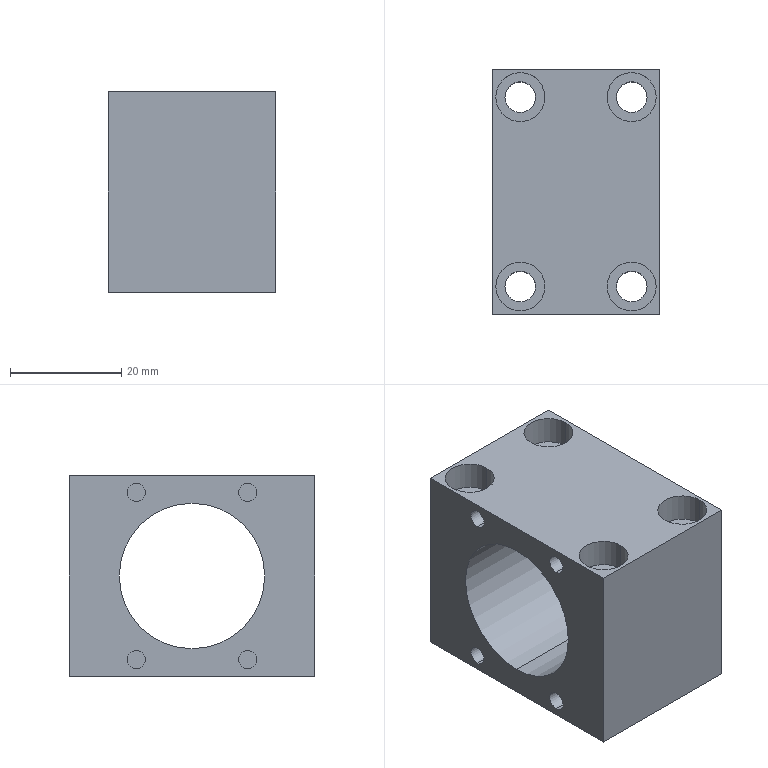Part | SolidWorks | features BaseBody 1 | 1 solid | 52 faces | box 30 x 44 x 36 mm | volume 26457 mm3 | cylinder 34 | plane 18 | commonest cylinder face diameters 3.3 x16 5.5 x8 8.8 x8 26.1 x2
STEP:
#1=CARTESIAN_POINT('',(-15.,0.,31.05));
#2=VERTEX_POINT('',#1);
#3=CARTESIAN_POINT('',(-15.,0.,4.95));
#4=VERTEX_POINT('',#3);
#5=CARTESIAN_POINT('',(-15.,0.,18.));
#6=DIRECTION('',(1.,0.,0.));
#7=DIRECTION('',(0.,0.,-1.));
#8=AXIS2_PLACEMENT_3D('',#5,#6,#7);
#9=CIRCLE('',#8,13.05);
#10=EDGE_CURVE('',#2,#4,#9,.T.);
#11=ORIENTED_EDGE('',*,*,#10,.F.);
#12=CARTESIAN_POINT('',(15.,0.,31.05));
#13=VERTEX_POINT('',#12);
#14=CARTESIAN_POINT('',(-16.,0.,31.05));
#15=DIRECTION('',(1.,0.,0.));
#16=VECTOR('',#15,1000.);
#17=LINE('',#14,#16);
#18=EDGE_CURVE('',#2,#13,#17,.T.);
#19=ORIENTED_EDGE('',*,*,#18,.T.);
#20=CARTESIAN_POINT('',(15.,0.,4.95));
#21=VERTEX_POINT('',#20);
#22=CARTESIAN_POINT('',(15.,0.,18.));
#23=DIRECTION('',(-1.,0.,0.));
#24=DIRECTION('',(0.,0.,-1.));
#25=AXIS2_PLACEMENT_3D('',#22,#23,#24);
#26=CIRCLE('',#25,13.05);
#27=EDGE_CURVE('',#21,#13,#26,.T.);
#28=ORIENTED_EDGE('',*,*,#27,.F.);
#29=CARTESIAN_POINT('',(-16.,0.,4.95));
#30=DIRECTION('',(1.,0.,0.));
#31=VECTOR('',#30,1000.);
#32=LINE('',#29,#31);
#33=EDGE_CURVE('',#4,#21,#32,.T.);
#34=ORIENTED_EDGE('',*,*,#33,.F.);
#35=EDGE_LOOP('',(#11,#19,#28,#34));
#36=FACE_OUTER_BOUND('',#35,.T.);
#37=CARTESIAN_POINT('',(-16.,0.,18.));
#38=DIRECTION('',(1.,0.,0.));
#39=DIRECTION('',(0.,0.,-1.));
#40=AXIS2_PLACEMENT_3D('',#37,#38,#39);
#41=CYLINDRICAL_SURFACE('',#40,13.05);
#42=ADVANCED_FACE('',(#36),#41,.F.);
#43=CARTESIAN_POINT('',(-2.8,-10.,31.35));
#44=VERTEX_POINT('',#43);
#45=CARTESIAN_POINT('',(-2.8,-10.,34.65));
#46=VERTEX_POINT('',#45);
#47=CARTESIAN_POINT('',(-2.8,-10.,33.));
#48=DIRECTION('',(-1.,0.,0.));
#49=DIRECTION('',(0.,0.,1.));
#50=AXIS2_PLACEMENT_3D('',#47,#48,#49);
#51=CIRCLE('',#50,1.65);
#52=EDGE_CURVE('',#44,#46,#51,.T.);
#53=ORIENTED_EDGE('',*,*,#52,.F.);
#54=CARTESIAN_POINT('',(-15.,-10.,31.35));
#55=VERTEX_POINT('',#54);
#56=CARTESIAN_POINT('',(-2.8,-10.,31.35));
#57=DIRECTION('',(-1.,0.,0.));
#58=VECTOR('',#57,1000.);
#59=LINE('',#56,#58);
#60=EDGE_CURVE('',#44,#55,#59,.T.);
#61=ORIENTED_EDGE('',*,*,#60,.T.);
#62=CARTESIAN_POINT('',(-15.,-10.,34.65));
#63=VERTEX_POINT('',#62);
#64=CARTESIAN_POINT('',(-15.,-10.,33.));
#65=DIRECTION('',(-1.,0.,0.));
#66=DIRECTION('',(0.,0.,1.));
#67=AXIS2_PLACEMENT_3D('',#64,#65,#66);
#68=CIRCLE('',#67,1.65);
#69=EDGE_CURVE('',#55,#63,#68,.T.);
#70=ORIENTED_EDGE('',*,*,#69,.T.);
#71=CARTESIAN_POINT('',(-2.8,-10.,34.65));
#72=DIRECTION('',(-1.,0.,0.));
#73=VECTOR('',#72,1000.);
#74=LINE('',#71,#73);
#75=EDGE_CURVE('',#46,#63,#74,.T.);
#76=ORIENTED_EDGE('',*,*,#75,.F.);
#77=EDGE_LOOP('',(#53,#61,#70,#76));
#78=FACE_OUTER_BOUND('',#77,.T.);
#79=CARTESIAN_POINT('',(-2.8,-10.,33.));
#80=DIRECTION('',(-1.,0.,0.));
#81=DIRECTION('',(0.,0.,1.));
#82=AXIS2_PLACEMENT_3D('',#79,#80,#81);
#83=CYLINDRICAL_SURFACE('',#82,1.65);
#84=ADVANCED_FACE('',(#78),#83,.F.);
#85=CARTESIAN_POINT('',(-2.8,-10.,1.35));
#86=VERTEX_POINT('',#85);
#87=CARTESIAN_POINT('',(-2.8,-10.,4.65));
#88=VERTEX_POINT('',#87);
#89=CARTESIAN_POINT('',(-2.8,-10.,3.));
#90=DIRECTION('',(-1.,0.,0.));
#91=DIRECTION('',(0.,0.,1.));
#92=AXIS2_PLACEMENT_3D('',#89,#90,#91);
#93=CIRCLE('',#92,1.65);
#94=EDGE_CURVE('',#86,#88,#93,.T.);
#95=ORIENTED_EDGE('',*,*,#94,.F.);
#96=CARTESIAN_POINT('',(-15.,-10.,1.35));
#97=VERTEX_POINT('',#96);
#98=CARTESIAN_POINT('',(-2.8,-10.,1.35));
#99=DIRECTION('',(-1.,0.,0.));
#100=VECTOR('',#99,1000.);
#101=LINE('',#98,#100);
#102=EDGE_CURVE('',#86,#97,#101,.T.);
#103=ORIENTED_EDGE('',*,*,#102,.T.);
#104=CARTESIAN_POINT('',(-15.,-10.,4.65));
#105=VERTEX_POINT('',#104);
#106=CARTESIAN_POINT('',(-15.,-10.,3.));
#107=DIRECTION('',(-1.,0.,0.));
#108=DIRECTION('',(0.,0.,1.));
#109=AXIS2_PLACEMENT_3D('',#106,#107,#108);
#110=CIRCLE('',#109,1.65);
#111=EDGE_CURVE('',#97,#105,#110,.T.);
#112=ORIENTED_EDGE('',*,*,#111,.T.);
#113=CARTESIAN_POINT('',(-2.8,-10.,4.65));
#114=DIRECTION('',(-1.,0.,0.));
#115=VECTOR('',#114,1000.);
#116=LINE('',#113,#115);
#117=EDGE_CURVE('',#88,#105,#116,.T.);
#118=ORIENTED_EDGE('',*,*,#117,.F.);
#119=EDGE_LOOP('',(#95,#103,#112,#118));
#120=FACE_OUTER_BOUND('',#119,.T.);
#121=CARTESIAN_POINT('',(-2.8,-10.,3.));
#122=DIRECTION('',(-1.,0.,0.));
#123=DIRECTION('',(0.,0.,1.));
#124=AXIS2_PLACEMENT_3D('',#121,#122,#123);
#125=CYLINDRICAL_SURFACE('',#124,1.65);
#126=ADVANCED_FACE('',(#120),#125,.F.);
#127=CARTESIAN_POINT('',(-2.8,10.,31.35));
#128=VERTEX_POINT('',#127);
#129=CARTESIAN_POINT('',(-2.8,10.,34.65));
#130=VERTEX_POINT('',#129);
#131=CARTESIAN_POINT('',(-2.8,10.,33.));
#132=DIRECTION('',(-1.,0.,0.));
#133=DIRECTION('',(0.,0.,1.));
#134=AXIS2_PLACEMENT_3D('',#131,#132,#133);
#135=CIRCLE('',#134,1.65);
#136=EDGE_CURVE('',#128,#130,#135,.T.);
#137=ORIENTED_EDGE('',*,*,#136,.F.);
#138=CARTESIAN_POINT('',(-15.,10.,31.35));
#139=VERTEX_POINT('',#138);
#140=CARTESIAN_POINT('',(-2.8,10.,31.35));
#141=DIRECTION('',(-1.,0.,0.));
#142=VECTOR('',#141,1000.);
#143=LINE('',#140,#142);
#144=EDGE_CURVE('',#128,#139,#143,.T.);
#145=ORIENTED_EDGE('',*,*,#144,.T.);
#146=CARTESIAN_POINT('',(-15.,10.,34.65));
#147=VERTEX_POINT('',#146);
#148=CARTESIAN_POINT('',(-15.,10.,33.));
#149=DIRECTION('',(-1.,0.,0.));
#150=DIRECTION('',(0.,0.,1.));
#151=AXIS2_PLACEMENT_3D('',#148,#149,#150);
#152=CIRCLE('',#151,1.65);
#153=EDGE_CURVE('',#139,#147,#152,.T.);
#154=ORIENTED_EDGE('',*,*,#153,.T.);
#155=CARTESIAN_POINT('',(-2.8,10.,34.65));
#156=DIRECTION('',(-1.,0.,0.));
#157=VECTOR('',#156,1000.);
#158=LINE('',#155,#157);
#159=EDGE_CURVE('',#130,#147,#158,.T.);
#160=ORIENTED_EDGE('',*,*,#159,.F.);
#161=EDGE_LOOP('',(#137,#145,#154,#160));
#162=FACE_OUTER_BOUND('',#161,.T.);
#163=CARTESIAN_POINT('',(-2.8,10.,33.));
#164=DIRECTION('',(-1.,0.,0.));
#165=DIRECTION('',(0.,0.,1.));
#166=AXIS2_PLACEMENT_3D('',#163,#164,#165);
#167=CYLINDRICAL_SURFACE('',#166,1.65);
#168=ADVANCED_FACE('',(#162),#167,.F.);
#169=CARTESIAN_POINT('',(-2.8,10.,1.35));
#170=VERTEX_POINT('',#169);
#171=CARTESIAN_POINT('',(-2.8,10.,4.65));
#172=VERTEX_POINT('',#171);
#173=CARTESIAN_POINT('',(-2.8,10.,3.));
#174=DIRECTION('',(-1.,0.,0.));
#175=DIRECTION('',(0.,0.,1.));
#176=AXIS2_PLACEMENT_3D('',#173,#174,#175);
#177=CIRCLE('',#176,1.65);
#178=EDGE_CURVE('',#170,#172,#177,.T.);
#179=ORIENTED_EDGE('',*,*,#178,.F.);
#180=CARTESIAN_POINT('',(-15.,10.,1.35));
#181=VERTEX_POINT('',#180);
#182=CARTESIAN_POINT('',(-2.8,10.,1.35));
#183=DIRECTION('',(-1.,0.,0.));
#184=VECTOR('',#183,1000.);
#185=LINE('',#182,#184);
#186=EDGE_CURVE('',#170,#181,#185,.T.);
#187=ORIENTED_EDGE('',*,*,#186,.T.);
#188=CARTESIAN_POINT('',(-15.,10.,4.65));
#189=VERTEX_POINT('',#188);
#190=CARTESIAN_POINT('',(-15.,10.,3.));
#191=DIRECTION('',(-1.,0.,0.));
#192=DIRECTION('',(0.,0.,1.));
#193=AXIS2_PLACEMENT_3D('',#190,#191,#192);
#194=CIRCLE('',#193,1.65);
#195=EDGE_CURVE('',#181,#189,#194,.T.);
#196=ORIENTED_EDGE('',*,*,#195,.T.);
#197=CARTESIAN_POINT('',(-2.8,10.,4.65));
#198=DIRECTION('',(-1.,0.,0.));
#199=VECTOR('',#198,1000.);
#200=LINE('',#197,#199);
#201=EDGE_CURVE('',#172,#189,#200,.T.);
#202=ORIENTED_EDGE('',*,*,#201,.F.);
#203=EDGE_LOOP('',(#179,#187,#196,#202));
#204=FACE_OUTER_BOUND('',#203,.T.);
#205=CARTESIAN_POINT('',(-2.8,10.,3.));
#206=DIRECTION('',(-1.,0.,0.));
#207=DIRECTION('',(0.,0.,1.));
#208=AXIS2_PLACEMENT_3D('',#205,#206,#207);
#209=CYLINDRICAL_SURFACE('',#208,1.65);
#210=ADVANCED_FACE('',(#204),#209,.F.);
#211=CARTESIAN_POINT('',(2.8,-10.,34.65));
#212=VERTEX_POINT('',#211);
#213=CARTESIAN_POINT('',(2.8,-10.,31.35));
#214=VERTEX_POINT('',#213);
#215=CARTESIAN_POINT('',(2.8,-10.,33.));
#216=DIRECTION('',(1.,0.,0.));
#217=DIRECTION('',(0.,0.,-1.));
#218=AXIS2_PLACEMENT_3D('',#215,#216,#217);
#219=CIRCLE('',#218,1.65);
#220=EDGE_CURVE('',#212,#214,#219,.T.);
#221=ORIENTED_EDGE('',*,*,#220,.F.);
#222=CARTESIAN_POINT('',(15.,-10.,34.65));
#223=VERTEX_POINT('',#222);
#224=CARTESIAN_POINT('',(2.8,-10.,34.65));
#225=DIRECTION('',(1.,0.,0.));
#226=VECTOR('',#225,1000.);
#227=LINE('',#224,#226);
#228=EDGE_CURVE('',#212,#223,#227,.T.);
#229=ORIENTED_EDGE('',*,*,#228,.T.);
#230=CARTESIAN_POINT('',(15.,-10.,31.35));
#231=VERTEX_POINT('',#230);
#232=CARTESIAN_POINT('',(15.,-10.,33.));
#233=DIRECTION('',(-1.,0.,0.));
#234=DIRECTION('',(0.,0.,-1.));
#235=AXIS2_PLACEMENT_3D('',#232,#233,#234);
#236=CIRCLE('',#235,1.65);
#237=EDGE_CURVE('',#231,#223,#236,.T.);
#238=ORIENTED_EDGE('',*,*,#237,.F.);
#239=CARTESIAN_POINT('',(2.8,-10.,31.35));
#240=DIRECTION('',(1.,0.,0.));
#241=VECTOR('',#240,1000.);
#242=LINE('',#239,#241);
#243=EDGE_CURVE('',#214,#231,#242,.T.);
#244=ORIENTED_EDGE('',*,*,#243,.F.);
#245=EDGE_LOOP('',(#221,#229,#238,#244));
#246=FACE_OUTER_BOUND('',#245,.T.);
#247=CARTESIAN_POINT('',(2.8,-10.,33.));
#248=DIRECTION('',(1.,0.,0.));
#249=DIRECTION('',(0.,0.,-1.));
#250=AXIS2_PLACEMENT_3D('',#247,#248,#249);
#251=CYLINDRICAL_SURFACE('',#250,1.65);
#252=ADVANCED_FACE('',(#246),#251,.F.);
#253=CARTESIAN_POINT('',(2.8,-10.,4.65));
#254=VERTEX_POINT('',#253);
#255=CARTESIAN_POINT('',(2.8,-10.,1.35));
#256=VERTEX_POINT('',#255);
#257=CARTESIAN_POINT('',(2.8,-10.,3.));
#258=DIRECTION('',(1.,0.,0.));
#259=DIRECTION('',(0.,0.,-1.));
#260=AXIS2_PLACEMENT_3D('',#257,#258,#259);
#261=CIRCLE('',#260,1.65);
#262=EDGE_CURVE('',#254,#256,#261,.T.);
#263=ORIENTED_EDGE('',*,*,#262,.F.);
#264=CARTESIAN_POINT('',(15.,-10.,4.65));
#265=VERTEX_POINT('',#264);
#266=CARTESIAN_POINT('',(2.8,-10.,4.65));
#267=DIRECTION('',(1.,0.,0.));
#268=VECTOR('',#267,1000.);
#269=LINE('',#266,#268);
#270=EDGE_CURVE('',#254,#265,#269,.T.);
#271=ORIENTED_EDGE('',*,*,#270,.T.);
#272=CARTESIAN_POINT('',(15.,-10.,1.35));
#273=VERTEX_POINT('',#272);
#274=CARTESIAN_POINT('',(15.,-10.,3.));
#275=DIRECTION('',(-1.,0.,0.));
#276=DIRECTION('',(0.,0.,-1.));
#277=AXIS2_PLACEMENT_3D('',#274,#275,#276);
#278=CIRCLE('',#277,1.65);
#279=EDGE_CURVE('',#273,#265,#278,.T.);
#280=ORIENTED_EDGE('',*,*,#279,.F.);
#281=CARTESIAN_POINT('',(2.8,-10.,1.35));
#282=DIRECTION('',(1.,0.,0.));
#283=VECTOR('',#282,1000.);
#284=LINE('',#281,#283);
#285=EDGE_CURVE('',#256,#273,#284,.T.);
#286=ORIENTED_EDGE('',*,*,#285,.F.);
#287=EDGE_LOOP('',(#263,#271,#280,#286));
#288=FACE_OUTER_BOUND('',#287,.T.);
#289=CARTESIAN_POINT('',(2.8,-10.,3.));
#290=DIRECTION('',(1.,0.,0.));
#291=DIRECTION('',(0.,0.,-1.));
#292=AXIS2_PLACEMENT_3D('',#289,#290,#291);
#293=CYLINDRICAL_SURFACE('',#292,1.65);
#294=ADVANCED_FACE('',(#288),#293,.F.);
#295=CARTESIAN_POINT('',(2.8,10.,34.65));
#296=VERTEX_POINT('',#295);
#297=CARTESIAN_POINT('',(2.8,10.,31.35));
#298=VERTEX_POINT('',#297);
#299=CARTESIAN_POINT('',(2.8,10.,33.));
#300=DIRECTION('',(1.,0.,0.));
#301=DIRECTION('',(0.,0.,-1.));
#302=AXIS2_PLACEMENT_3D('',#299,#300,#301);
#303=CIRCLE('',#302,1.65);
#304=EDGE_CURVE('',#296,#298,#303,.T.);
#305=ORIENTED_EDGE('',*,*,#304,.F.);
#306=CARTESIAN_POINT('',(15.,10.,34.65));
#307=VERTEX_POINT('',#306);
#308=CARTESIAN_POINT('',(2.8,10.,34.65));
#309=DIRECTION('',(1.,0.,0.));
#310=VECTOR('',#309,1000.);
#311=LINE('',#308,#310);
#312=EDGE_CURVE('',#296,#307,#311,.T.);
#313=ORIENTED_EDGE('',*,*,#312,.T.);
#314=CARTESIAN_POINT('',(15.,10.,31.35));
#315=VERTEX_POINT('',#314);
#316=CARTESIAN_POINT('',(15.,10.,33.));
#317=DIRECTION('',(-1.,0.,0.));
#318=DIRECTION('',(0.,0.,-1.));
#319=AXIS2_PLACEMENT_3D('',#316,#317,#318);
#320=CIRCLE('',#319,1.65);
#321=EDGE_CURVE('',#315,#307,#320,.T.);
#322=ORIENTED_EDGE('',*,*,#321,.F.);
#323=CARTESIAN_POINT('',(2.8,10.,31.35));
#324=DIRECTION('',(1.,0.,0.));
#325=VECTOR('',#324,1000.);
#326=LINE('',#323,#325);
#327=EDGE_CURVE('',#298,#315,#326,.T.);
#328=ORIENTED_EDGE('',*,*,#327,.F.);
#329=EDGE_LOOP('',(#305,#313,#322,#328));
#330=FACE_OUTER_BOUND('',#329,.T.);
#331=CARTESIAN_POINT('',(2.8,10.,33.));
#332=DIRECTION('',(1.,0.,0.));
#333=DIRECTION('',(0.,0.,-1.));
#334=AXIS2_PLACEMENT_3D('',#331,#332,#333);
#335=CYLINDRICAL_SURFACE('',#334,1.65);
#336=ADVANCED_FACE('',(#330),#335,.F.);
#337=CARTESIAN_POINT('',(2.8,10.,4.65));
#338=VERTEX_POINT('',#337);
#339=CARTESIAN_POINT('',(2.8,10.,1.35));
#340=VERTEX_POINT('',#339);
#341=CARTESIAN_POINT('',(2.8,10.,3.));
#342=DIRECTION('',(1.,0.,0.));
#343=DIRECTION('',(0.,0.,-1.));
#344=AXIS2_PLACEMENT_3D('',#341,#342,#343);
#345=CIRCLE('',#344,1.65);
#346=EDGE_CURVE('',#338,#340,#345,.T.);
#347=ORIENTED_EDGE('',*,*,#346,.F.);
#348=CARTESIAN_POINT('',(15.,10.,4.65));
#349=VERTEX_POINT('',#348);
#350=CARTESIAN_POINT('',(2.8,10.,4.65));
#351=DIRECTION('',(1.,0.,0.));
#352=VECTOR('',#351,1000.);
#353=LINE('',#350,#352);
#354=EDGE_CURVE('',#338,#349,#353,.T.);
#355=ORIENTED_EDGE('',*,*,#354,.T.);
#356=CARTESIAN_POINT('',(15.,10.,1.35));
#357=VERTEX_POINT('',#356);
#358=CARTESIAN_POINT('',(15.,10.,3.));
#359=DIRECTION('',(-1.,0.,0.));
#360=DIRECTION('',(0.,0.,-1.));
#361=AXIS2_PLACEMENT_3D('',#358,#359,#360);
#362=CIRCLE('',#361,1.65);
#363=EDGE_CURVE('',#357,#349,#362,.T.);
#364=ORIENTED_EDGE('',*,*,#363,.F.);
#365=CARTESIAN_POINT('',(2.8,10.,1.35));
#366=DIRECTION('',(1.,0.,0.));
#367=VECTOR('',#366,1000.);
#368=LINE('',#365,#367);
#369=EDGE_CURVE('',#340,#357,#368,.T.);
#370=ORIENTED_EDGE('',*,*,#369,.F.);
#371=EDGE_LOOP('',(#347,#355,#364,#370));
#372=FACE_OUTER_BOUND('',#371,.T.);
#373=CARTESIAN_POINT('',(2.8,10.,3.));
#374=DIRECTION('',(1.,0.,0.));
#375=DIRECTION('',(0.,0.,-1.));
#376=AXIS2_PLACEMENT_3D('',#373,#374,#375);
#377=CYLINDRICAL_SURFACE('',#376,1.65);
#378=ADVANCED_FACE('',(#372),#377,.F.);
#379=CARTESIAN_POINT('',(5.6,17.,30.9));
#380=VERTEX_POINT('',#379);
#381=CARTESIAN_POINT('',(14.4,17.,30.9));
#382=VERTEX_POINT('',#381);
#383=CARTESIAN_POINT('',(10.,17.,30.9));
#384=DIRECTION('',(0.,0.,1.));
#385=DIRECTION('',(1.,0.,0.));
#386=AXIS2_PLACEMENT_3D('',#383,#384,#385);
#387=CIRCLE('',#386,4.4);
#388=EDGE_CURVE('',#380,#382,#387,.T.);
#389=ORIENTED_EDGE('',*,*,#388,.F.);
#390=CARTESIAN_POINT('',(5.6,17.,36.));
#391=VERTEX_POINT('',#390);
#392=CARTESIAN_POINT('',(5.6,17.,30.9));
#393=DIRECTION('',(0.,0.,1.));
#394=VECTOR('',#393,1000.);
#395=LINE('',#392,#394);
#396=EDGE_CURVE('',#380,#391,#395,.T.);
#397=ORIENTED_EDGE('',*,*,#396,.T.);
#398=CARTESIAN_POINT('',(14.4,17.,36.));
#399=VERTEX_POINT('',#398);
#400=CARTESIAN_POINT('',(10.,17.,36.));
#401=DIRECTION('',(0.,0.,-1.));
#402=DIRECTION('',(1.,0.,0.));
#403=AXIS2_PLACEMENT_3D('',#400,#401,#402);
#404=CIRCLE('',#403,4.4);
#405=EDGE_CURVE('',#399,#391,#404,.T.);
#406=ORIENTED_EDGE('',*,*,#405,.F.);
#407=CARTESIAN_POINT('',(14.4,17.,30.9));
#408=DIRECTION('',(0.,0.,1.));
#409=VECTOR('',#408,1000.);
#410=LINE('',#407,#409);
#411=EDGE_CURVE('',#382,#399,#410,.T.);
#412=ORIENTED_EDGE('',*,*,#411,.F.);
#413=EDGE_LOOP('',(#389,#397,#406,#412));
#414=FACE_OUTER_BOUND('',#413,.T.);
#415=CARTESIAN_POINT('',(10.,17.,30.9));
#416=DIRECTION('',(0.,0.,1.));
#417=DIRECTION('',(1.,0.,0.));
#418=AXIS2_PLACEMENT_3D('',#415,#416,#417);
#419=CYLINDRICAL_SURFACE('',#418,4.4);
#420=ADVANCED_FACE('',(#414),#419,.F.);
#421=CARTESIAN_POINT('',(-14.4,17.,30.9));
#422=VERTEX_POINT('',#421);
#423=CARTESIAN_POINT('',(-5.6,17.,30.9));
#424=VERTEX_POINT('',#423);
#425=CARTESIAN_POINT('',(-10.,17.,30.9));
#426=DIRECTION('',(0.,0.,1.));
#427=DIRECTION('',(1.,0.,0.));
#428=AXIS2_PLACEMENT_3D('',#425,#426,#427);
#429=CIRCLE('',#428,4.4);
#430=EDGE_CURVE('',#422,#424,#429,.T.);
#431=ORIENTED_EDGE('',*,*,#430,.F.);
#432=CARTESIAN_POINT('',(-14.4,17.,36.));
#433=VERTEX_POINT('',#432);
#434=CARTESIAN_POINT('',(-14.4,17.,30.9));
#435=DIRECTION('',(0.,0.,1.));
#436=VECTOR('',#435,1000.);
#437=LINE('',#434,#436);
#438=EDGE_CURVE('',#422,#433,#437,.T.);
#439=ORIENTED_EDGE('',*,*,#438,.T.);
#440=CARTESIAN_POINT('',(-5.6,17.,36.));
#441=VERTEX_POINT('',#440);
#442=CARTESIAN_POINT('',(-10.,17.,36.));
#443=DIRECTION('',(0.,0.,-1.));
#444=DIRECTION('',(1.,0.,0.));
#445=AXIS2_PLACEMENT_3D('',#442,#443,#444);
#446=CIRCLE('',#445,4.4);
#447=EDGE_CURVE('',#441,#433,#446,.T.);
#448=ORIENTED_EDGE('',*,*,#447,.F.);
#449=CARTESIAN_POINT('',(-5.6,17.,30.9));
#450=DIRECTION('',(0.,0.,1.));
#451=VECTOR('',#450,1000.);
#452=LINE('',#449,#451);
#453=EDGE_CURVE('',#424,#441,#452,.T.);
#454=ORIENTED_EDGE('',*,*,#453,.F.);
#455=EDGE_LOOP('',(#431,#439,#448,#454));
#456=FACE_OUTER_BOUND('',#455,.T.);
#457=CARTESIAN_POINT('',(-10.,17.,30.9));
#458=DIRECTION('',(0.,0.,1.));
#459=DIRECTION('',(1.,0.,0.));
#460=AXIS2_PLACEMENT_3D('',#457,#458,#459);
#461=CYLINDRICAL_SURFACE('',#460,4.4);
#462=ADVANCED_FACE('',(#456),#461,.F.);
#463=CARTESIAN_POINT('',(5.6,-17.,30.9));
#464=VERTEX_POINT('',#463);
#465=CARTESIAN_POINT('',(14.4,-17.,30.9));
#466=VERTEX_POINT('',#465);
#467=CARTESIAN_POINT('',(10.,-17.,30.9));
#468=DIRECTION('',(0.,0.,1.));
#469=DIRECTION('',(1.,0.,0.));
#470=AXIS2_PLACEMENT_3D('',#467,#468,#469);
#471=CIRCLE('',#470,4.4);
#472=EDGE_CURVE('',#464,#466,#471,.T.);
#473=ORIENTED_EDGE('',*,*,#472,.F.);
#474=CARTESIAN_POINT('',(5.6,-17.,36.));
#475=VERTEX_POINT('',#474);
#476=CARTESIAN_POINT('',(5.6,-17.,30.9));
#477=DIRECTION('',(0.,0.,1.));
#478=VECTOR('',#477,1000.);
#479=LINE('',#476,#478);
#480=EDGE_CURVE('',#464,#475,#479,.T.);
#481=ORIENTED_EDGE('',*,*,#480,.T.);
#482=CARTESIAN_POINT('',(14.4,-17.,36.));
#483=VERTEX_POINT('',#482);
#484=CARTESIAN_POINT('',(10.,-17.,36.));
#485=DIRECTION('',(0.,0.,-1.));
#486=DIRECTION('',(1.,0.,0.));
#487=AXIS2_PLACEMENT_3D('',#484,#485,#486);
#488=CIRCLE('',#487,4.4);
#489=EDGE_CURVE('',#483,#475,#488,.T.);
#490=ORIENTED_EDGE('',*,*,#489,.F.);
#491=CARTESIAN_POINT('',(14.4,-17.,30.9));
#492=DIRECTION('',(0.,0.,1.));
#493=VECTOR('',#492,1000.);
#494=LINE('',#491,#493);
#495=EDGE_CURVE('',#466,#483,#494,.T.);
#496=ORIENTED_EDGE('',*,*,#495,.F.);
#497=EDGE_LOOP('',(#473,#481,#490,#496));
#498=FACE_OUTER_BOUND('',#497,.T.);
#499=CARTESIAN_POINT('',(10.,-17.,30.9));
#500=DIRECTION('',(0.,0.,1.));
#501=DIRECTION('',(1.,0.,0.));
#502=AXIS2_PLACEMENT_3D('',#499,#500,#501);
#503=CYLINDRICAL_SURFACE('',#502,4.4);
#504=ADVANCED_FACE('',(#498),#503,.F.);
#505=CARTESIAN_POINT('',(-14.4,-17.,30.9));
#506=VERTEX_POINT('',#505);
#507=CARTESIAN_POINT('',(-5.6,-17.,30.9));
#508=VERTEX_POINT('',#507);
#509=CARTESIAN_POINT('',(-10.,-17.,30.9));
#510=DIRECTION('',(0.,0.,1.));
#511=DIRECTION('',(1.,0.,0.));
#512=AXIS2_PLACEMENT_3D('',#509,#510,#511);
#513=CIRCLE('',#512,4.4);
#514=EDGE_CURVE('',#506,#508,#513,.T.);
#515=ORIENTED_EDGE('',*,*,#514,.F.);
#516=CARTESIAN_POINT('',(-14.4,-17.,36.));
#517=VERTEX_POINT('',#516);
#518=CARTESIAN_POINT('',(-14.4,-17.,30.9));
#519=DIRECTION('',(0.,0.,1.));
#520=VECTOR('',#519,1000.);
#521=LINE('',#518,#520);
#522=EDGE_CURVE('',#506,#517,#521,.T.);
#523=ORIENTED_EDGE('',*,*,#522,.T.);
#524=CARTESIAN_POINT('',(-5.6,-17.,36.));
#525=VERTEX_POINT('',#524);
#526=CARTESIAN_POINT('',(-10.,-17.,36.));
#527=DIRECTION('',(0.,0.,-1.));
#528=DIRECTION('',(1.,0.,0.));
#529=AXIS2_PLACEMENT_3D('',#526,#527,#528);
#530=CIRCLE('',#529,4.4);
#531=EDGE_CURVE('',#525,#517,#530,.T.);
#532=ORIENTED_EDGE('',*,*,#531,.F.);
#533=CARTESIAN_POINT('',(-5.6,-17.,30.9));
#534=DIRECTION('',(0.,0.,1.));
#535=VECTOR('',#534,1000.);
#536=LINE('',#533,#535);
#537=EDGE_CURVE('',#508,#525,#536,.T.);
#538=ORIENTED_EDGE('',*,*,#537,.F.);
#539=EDGE_LOOP('',(#515,#523,#532,#538));
#540=FACE_OUTER_BOUND('',#539,.T.);
#541=CARTESIAN_POINT('',(-10.,-17.,30.9));
#542=DIRECTION('',(0.,0.,1.));
#543=DIRECTION('',(1.,0.,0.));
#544=AXIS2_PLACEMENT_3D('',#541,#542,#543);
#545=CYLINDRICAL_SURFACE('',#544,4.4);
#546=ADVANCED_FACE('',(#540),#545,.F.);
#547=CARTESIAN_POINT('',(12.75,17.,0.));
#548=VERTEX_POINT('',#547);
#549=CARTESIAN_POINT('',(7.25,17.,0.));
#550=VERTEX_POINT('',#549);
#551=CARTESIAN_POINT('',(10.,17.,0.));
#552=DIRECTION('',(0.,0.,-1.));
#553=DIRECTION('',(1.,0.,0.));
#554=AXIS2_PLACEMENT_3D('',#551,#552,#553);
#555=CIRCLE('',#554,2.75);
#556=EDGE_CURVE('',#548,#550,#555,.T.);
#557=ORIENTED_EDGE('',*,*,#556,.T.);
#558=CARTESIAN_POINT('',(7.25,17.,30.9));
#559=VERTEX_POINT('',#558);
#560=CARTESIAN_POINT('',(7.25,17.,-1.));
#561=DIRECTION('',(0.,0.,1.));
#562=VECTOR('',#561,1000.);
#563=LINE('',#560,#562);
#564=EDGE_CURVE('',#550,#559,#563,.T.);
#565=ORIENTED_EDGE('',*,*,#564,.T.);
#566=CARTESIAN_POINT('',(12.75,17.,30.9));
#567=VERTEX_POINT('',#566);
#568=CARTESIAN_POINT('',(10.,17.,30.9));
#569=DIRECTION('',(0.,0.,-1.));
#570=DIRECTION('',(1.,0.,0.));
#571=AXIS2_PLACEMENT_3D('',#568,#569,#570);
#572=CIRCLE('',#571,2.75);
#573=EDGE_CURVE('',#567,#559,#572,.T.);
#574=ORIENTED_EDGE('',*,*,#573,.F.);
#575=CARTESIAN_POINT('',(12.75,17.,-1.));
#576=DIRECTION('',(0.,0.,1.));
#577=VECTOR('',#576,1000.);
#578=LINE('',#575,#577);
#579=EDGE_CURVE('',#548,#567,#578,.T.);
#580=ORIENTED_EDGE('',*,*,#579,.F.);
#581=EDGE_LOOP('',(#557,#565,#574,#580));
#582=FACE_OUTER_BOUND('',#581,.T.);
#583=CARTESIAN_POINT('',(10.,17.,-1.));
#584=DIRECTION('',(0.,0.,1.));
#585=DIRECTION('',(1.,0.,0.));
#586=AXIS2_PLACEMENT_3D('',#583,#584,#585);
#587=CYLINDRICAL_SURFACE('',#586,2.75);
#588=ADVANCED_FACE('',(#582),#587,.F.);
#589=CARTESIAN_POINT('',(-7.25,17.,0.));
#590=VERTEX_POINT('',#589);
#591=CARTESIAN_POINT('',(-12.75,17.,0.));
#592=VERTEX_POINT('',#591);
#593=CARTESIAN_POINT('',(-10.,17.,0.));
#594=DIRECTION('',(0.,0.,-1.));
#595=DIRECTION('',(1.,0.,0.));
#596=AXIS2_PLACEMENT_3D('',#593,#594,#595);
#597=CIRCLE('',#596,2.75);
#598=EDGE_CURVE('',#590,#592,#597,.T.);
#599=ORIENTED_EDGE('',*,*,#598,.T.);
#600=CARTESIAN_POINT('',(-12.75,17.,30.9));
#601=VERTEX_POINT('',#600);
#602=CARTESIAN_POINT('',(-12.75,17.,-1.));
#603=DIRECTION('',(0.,0.,1.));
#604=VECTOR('',#603,1000.);
#605=LINE('',#602,#604);
#606=EDGE_CURVE('',#592,#601,#605,.T.);
#607=ORIENTED_EDGE('',*,*,#606,.T.);
#608=CARTESIAN_POINT('',(-7.25,17.,30.9));
#609=VERTEX_POINT('',#608);
#610=CARTESIAN_POINT('',(-10.,17.,30.9));
#611=DIRECTION('',(0.,0.,-1.));
#612=DIRECTION('',(1.,0.,0.));
#613=AXIS2_PLACEMENT_3D('',#610,#611,#612);
#614=CIRCLE('',#613,2.75);
#615=EDGE_CURVE('',#609,#601,#614,.T.);
#616=ORIENTED_EDGE('',*,*,#615,.F.);
#617=CARTESIAN_POINT('',(-7.25,17.,-1.));
#618=DIRECTION('',(0.,0.,1.));
#619=VECTOR('',#618,1000.);
#620=LINE('',#617,#619);
#621=EDGE_CURVE('',#590,#609,#620,.T.);
#622=ORIENTED_EDGE('',*,*,#621,.F.);
#623=EDGE_LOOP('',(#599,#607,#616,#622));
#624=FACE_OUTER_BOUND('',#623,.T.);
#625=CARTESIAN_POINT('',(-10.,17.,-1.));
#626=DIRECTION('',(0.,0.,1.));
#627=DIRECTION('',(1.,0.,0.));
#628=AXIS2_PLACEMENT_3D('',#625,#626,#627);
#629=CYLINDRICAL_SURFACE('',#628,2.75);
#630=ADVANCED_FACE('',(#624),#629,.F.);
#631=CARTESIAN_POINT('',(12.75,-17.,0.));
#632=VERTEX_POINT('',#631);
#633=CARTESIAN_POINT('',(7.25,-17.,0.));
#634=VERTEX_POINT('',#633);
#635=CARTESIAN_POINT('',(10.,-17.,0.));
#636=DIRECTION('',(0.,0.,-1.));
#637=DIRECTION('',(1.,0.,0.));
#638=AXIS2_PLACEMENT_3D('',#635,#636,#637);
#639=CIRCLE('',#638,2.75);
#640=EDGE_CURVE('',#632,#634,#639,.T.);
#641=ORIENTED_EDGE('',*,*,#640,.T.);
#642=CARTESIAN_POINT('',(7.25,-17.,30.9));
#643=VERTEX_POINT('',#642);
#644=CARTESIAN_POINT('',(7.25,-17.,-1.));
#645=DIRECTION('',(0.,0.,1.));
#646=VECTOR('',#645,1000.);
#647=LINE('',#644,#646);
#648=EDGE_CURVE('',#634,#643,#647,.T.);
#649=ORIENTED_EDGE('',*,*,#648,.T.);
#650=CARTESIAN_POINT('',(12.75,-17.,30.9));
#651=VERTEX_POINT('',#650);
#652=CARTESIAN_POINT('',(10.,-17.,30.9));
#653=DIRECTION('',(0.,0.,-1.));
#654=DIRECTION('',(1.,0.,0.));
#655=AXIS2_PLACEMENT_3D('',#652,#653,#654);
#656=CIRCLE('',#655,2.75);
#657=EDGE_CURVE('',#651,#643,#656,.T.);
#658=ORIENTED_EDGE('',*,*,#657,.F.);
#659=CARTESIAN_POINT('',(12.75,-17.,-1.));
#660=DIRECTION('',(0.,0.,1.));
#661=VECTOR('',#660,1000.);
#662=LINE('',#659,#661);
#663=EDGE_CURVE('',#632,#651,#662,.T.);
#664=ORIENTED_EDGE('',*,*,#663,.F.);
#665=EDGE_LOOP('',(#641,#649,#658,#664));
#666=FACE_OUTER_BOUND('',#665,.T.);
#667=CARTESIAN_POINT('',(10.,-17.,-1.));
#668=DIRECTION('',(0.,0.,1.));
#669=DIRECTION('',(1.,0.,0.));
#670=AXIS2_PLACEMENT_3D('',#667,#668,#669);
#671=CYLINDRICAL_SURFACE('',#670,2.75);
#672=ADVANCED_FACE('',(#666),#671,.F.);
#673=CARTESIAN_POINT('',(-7.25,-17.,0.));
#674=VERTEX_POINT('',#673);
#675=CARTESIAN_POINT('',(-12.75,-17.,0.));
#676=VERTEX_POINT('',#675);
#677=CARTESIAN_POINT('',(-10.,-17.,0.));
#678=DIRECTION('',(0.,0.,-1.));
#679=DIRECTION('',(1.,0.,0.));
#680=AXIS2_PLACEMENT_3D('',#677,#678,#679);
#681=CIRCLE('',#680,2.75);
#682=EDGE_CURVE('',#674,#676,#681,.T.);
#683=ORIENTED_EDGE('',*,*,#682,.T.);
#684=CARTESIAN_POINT('',(-12.75,-17.,30.9));
#685=VERTEX_POINT('',#684);
#686=CARTESIAN_POINT('',(-12.75,-17.,-1.));
#687=DIRECTION('',(0.,0.,1.));
#688=VECTOR('',#687,1000.);
#689=LINE('',#686,#688);
#690=EDGE_CURVE('',#676,#685,#689,.T.);
#691=ORIENTED_EDGE('',*,*,#690,.T.);
#692=CARTESIAN_POINT('',(-7.25,-17.,30.9));
#693=VERTEX_POINT('',#692);
#694=CARTESIAN_POINT('',(-10.,-17.,30.9));
#695=DIRECTION('',(0.,0.,-1.));
#696=DIRECTION('',(1.,0.,0.));
#697=AXIS2_PLACEMENT_3D('',#694,#695,#696);
#698=CIRCLE('',#697,2.75);
#699=EDGE_CURVE('',#693,#685,#698,.T.);
#700=ORIENTED_EDGE('',*,*,#699,.F.);
#701=CARTESIAN_POINT('',(-7.25,-17.,-1.));
#702=DIRECTION('',(0.,0.,1.));
#703=VECTOR('',#702,1000.);
#704=LINE('',#701,#703);
#705=EDGE_CURVE('',#674,#693,#704,.T.);
#706=ORIENTED_EDGE('',*,*,#705,.F.);
#707=EDGE_LOOP('',(#683,#691,#700,#706));
#708=FACE_OUTER_BOUND('',#707,.T.);
#709=CARTESIAN_POINT('',(-10.,-17.,-1.));
#710=DIRECTION('',(0.,0.,1.));
#711=DIRECTION('',(1.,0.,0.));
#712=AXIS2_PLACEMENT_3D('',#709,#710,#711);
#713=CYLINDRICAL_SURFACE('',#712,2.75);
#714=ADVANCED_FACE('',(#708),#713,.F.);
#715=ORIENTED_EDGE('',*,*,#18,.F.);
#716=CARTESIAN_POINT('',(-15.,0.,18.));
#717=DIRECTION('',(1.,0.,0.));
#718=DIRECTION('',(0.,0.,-1.));
#719=AXIS2_PLACEMENT_3D('',#716,#717,#718);
#720=CIRCLE('',#719,13.05);
#721=EDGE_CURVE('',#4,#2,#720,.T.);
#722=ORIENTED_EDGE('',*,*,#721,.F.);
#723=ORIENTED_EDGE('',*,*,#33,.T.);
#724=CARTESIAN_POINT('',(15.,0.,18.));
#725=DIRECTION('',(-1.,0.,0.));
#726=DIRECTION('',(0.,0.,-1.));
#727=AXIS2_PLACEMENT_3D('',#724,#725,#726);
#728=CIRCLE('',#727,13.05);
#729=EDGE_CURVE('',#13,#21,#728,.T.);
#730=ORIENTED_EDGE('',*,*,#729,.F.);
#731=EDGE_LOOP('',(#715,#722,#723,#730));
#732=FACE_OUTER_BOUND('',#731,.T.);
#733=CARTESIAN_POINT('',(-16.,0.,18.));
#734=DIRECTION('',(1.,0.,0.));
#735=DIRECTION('',(0.,0.,-1.));
#736=AXIS2_PLACEMENT_3D('',#733,#734,#735);
#737=CYLINDRICAL_SURFACE('',#736,13.05);
#738=ADVANCED_FACE('',(#732),#737,.F.);
#739=CARTESIAN_POINT('',(-15.,-10.,33.));
#740=DIRECTION('',(-1.,0.,0.));
#741=DIRECTION('',(0.,0.,1.));
#742=AXIS2_PLACEMENT_3D('',#739,#740,#741);
#743=CIRCLE('',#742,1.65);
#744=EDGE_CURVE('',#63,#55,#743,.T.);
#745=ORIENTED_EDGE('',*,*,#744,.F.);
#746=ORIENTED_EDGE('',*,*,#69,.F.);
#747=EDGE_LOOP('',(#745,#746));
#748=FACE_BOUND('',#747,.T.);
#749=CARTESIAN_POINT('',(-15.,-10.,3.));
#750=DIRECTION('',(-1.,0.,0.));
#751=DIRECTION('',(0.,0.,1.));
#752=AXIS2_PLACEMENT_3D('',#749,#750,#751);
#753=CIRCLE('',#752,1.65);
#754=EDGE_CURVE('',#105,#97,#753,.T.);
#755=ORIENTED_EDGE('',*,*,#754,.F.);
#756=ORIENTED_EDGE('',*,*,#111,.F.);
#757=EDGE_LOOP('',(#755,#756));
#758=FACE_BOUND('',#757,.T.);
#759=ORIENTED_EDGE('',*,*,#721,.T.);
#760=ORIENTED_EDGE('',*,*,#10,.T.);
#761=EDGE_LOOP('',(#759,#760));
#762=FACE_BOUND('',#761,.T.);
#763=CARTESIAN_POINT('',(-15.,10.,33.));
#764=DIRECTION('',(-1.,0.,0.));
#765=DIRECTION('',(0.,0.,1.));
#766=AXIS2_PLACEMENT_3D('',#763,#764,#765);
#767=CIRCLE('',#766,1.65);
#768=EDGE_CURVE('',#147,#139,#767,.T.);
#769=ORIENTED_EDGE('',*,*,#768,.F.);
#770=ORIENTED_EDGE('',*,*,#153,.F.);
#771=EDGE_LOOP('',(#769,#770));
#772=FACE_BOUND('',#771,.T.);
#773=CARTESIAN_POINT('',(-15.,10.,3.));
#774=DIRECTION('',(-1.,0.,0.));
#775=DIRECTION('',(0.,0.,1.));
#776=AXIS2_PLACEMENT_3D('',#773,#774,#775);
#777=CIRCLE('',#776,1.65);
#778=EDGE_CURVE('',#189,#181,#777,.T.);
#779=ORIENTED_EDGE('',*,*,#778,.F.);
#780=ORIENTED_EDGE('',*,*,#195,.F.);
#781=EDGE_LOOP('',(#779,#780));
#782=FACE_BOUND('',#781,.T.);
#783=CARTESIAN_POINT('',(-15.,22.,0.));
#784=VERTEX_POINT('',#783);
#785=CARTESIAN_POINT('',(-15.,22.,36.));
#786=VERTEX_POINT('',#785);
#787=CARTESIAN_POINT('',(-15.,22.,0.));
#788=DIRECTION('',(0.,0.,1.));
#789=VECTOR('',#788,1000.);
#790=LINE('',#787,#789);
#791=EDGE_CURVE('',#784,#786,#790,.T.);
#792=ORIENTED_EDGE('',*,*,#791,.F.);
#793=CARTESIAN_POINT('',(-15.,-22.,0.));
#794=VERTEX_POINT('',#793);
#795=CARTESIAN_POINT('',(-15.,-22.,0.));
#796=DIRECTION('',(0.,1.,0.));
#797=VECTOR('',#796,1000.);
#798=LINE('',#795,#797);
#799=EDGE_CURVE('',#794,#784,#798,.T.);
#800=ORIENTED_EDGE('',*,*,#799,.F.);
#801=CARTESIAN_POINT('',(-15.,-22.,36.));
#802=VERTEX_POINT('',#801);
#803=CARTESIAN_POINT('',(-15.,-22.,0.));
#804=DIRECTION('',(0.,0.,-1.));
#805=VECTOR('',#804,1000.);
#806=LINE('',#803,#805);
#807=EDGE_CURVE('',#802,#794,#806,.T.);
#808=ORIENTED_EDGE('',*,*,#807,.F.);
#809=CARTESIAN_POINT('',(-15.,-22.,36.));
#810=DIRECTION('',(0.,-1.,0.));
#811=VECTOR('',#810,1000.);
#812=LINE('',#809,#811);
#813=EDGE_CURVE('',#786,#802,#812,.T.);
#814=ORIENTED_EDGE('',*,*,#813,.F.);
#815=EDGE_LOOP('',(#792,#800,#808,#814));
#816=FACE_OUTER_BOUND('',#815,.T.);
#817=CARTESIAN_POINT('',(-15.,-22.,0.));
#818=DIRECTION('',(1.,0.,0.));
#819=DIRECTION('',(0.,0.,-1.));
#820=AXIS2_PLACEMENT_3D('',#817,#818,#819);
#821=PLANE('',#820);
#822=ADVANCED_FACE('',(#748,#758,#762,#772,#782,#816),#821,.F.);
#823=ORIENTED_EDGE('',*,*,#237,.T.);
#824=CARTESIAN_POINT('',(15.,-10.,33.));
#825=DIRECTION('',(-1.,0.,0.));
#826=DIRECTION('',(0.,0.,-1.));
#827=AXIS2_PLACEMENT_3D('',#824,#825,#826);
#828=CIRCLE('',#827,1.65);
#829=EDGE_CURVE('',#223,#231,#828,.T.);
#830=ORIENTED_EDGE('',*,*,#829,.T.);
#831=EDGE_LOOP('',(#823,#830));
#832=FACE_BOUND('',#831,.T.);
#833=ORIENTED_EDGE('',*,*,#279,.T.);
#834=CARTESIAN_POINT('',(15.,-10.,3.));
#835=DIRECTION('',(-1.,0.,0.));
#836=DIRECTION('',(0.,0.,-1.));
#837=AXIS2_PLACEMENT_3D('',#834,#835,#836);
#838=CIRCLE('',#837,1.65);
#839=EDGE_CURVE('',#265,#273,#838,.T.);
#840=ORIENTED_EDGE('',*,*,#839,.T.);
#841=EDGE_LOOP('',(#833,#840));
#842=FACE_BOUND('',#841,.T.);
#843=ORIENTED_EDGE('',*,*,#27,.T.);
#844=ORIENTED_EDGE('',*,*,#729,.T.);
#845=EDGE_LOOP('',(#843,#844));
#846=FACE_BOUND('',#845,.T.);
#847=ORIENTED_EDGE('',*,*,#321,.T.);
#848=CARTESIAN_POINT('',(15.,10.,33.));
#849=DIRECTION('',(-1.,0.,0.));
#850=DIRECTION('',(0.,0.,-1.));
#851=AXIS2_PLACEMENT_3D('',#848,#849,#850);
#852=CIRCLE('',#851,1.65);
#853=EDGE_CURVE('',#307,#315,#852,.T.);
#854=ORIENTED_EDGE('',*,*,#853,.T.);
#855=EDGE_LOOP('',(#847,#854));
#856=FACE_BOUND('',#855,.T.);
#857=ORIENTED_EDGE('',*,*,#363,.T.);
#858=CARTESIAN_POINT('',(15.,10.,3.));
#859=DIRECTION('',(-1.,0.,0.));
#860=DIRECTION('',(0.,0.,-1.));
#861=AXIS2_PLACEMENT_3D('',#858,#859,#860);
#862=CIRCLE('',#861,1.65);
#863=EDGE_CURVE('',#349,#357,#862,.T.);
#864=ORIENTED_EDGE('',*,*,#863,.T.);
#865=EDGE_LOOP('',(#857,#864));
#866=FACE_BOUND('',#865,.T.);
#867=CARTESIAN_POINT('',(15.,22.,0.));
#868=VERTEX_POINT('',#867);
#869=CARTESIAN_POINT('',(15.,22.,36.));
#870=VERTEX_POINT('',#869);
#871=CARTESIAN_POINT('',(15.,22.,0.));
#872=DIRECTION('',(0.,0.,1.));
#873=VECTOR('',#872,1000.);
#874=LINE('',#871,#873);
#875=EDGE_CURVE('',#868,#870,#874,.T.);
#876=ORIENTED_EDGE('',*,*,#875,.T.);
#877=CARTESIAN_POINT('',(15.,-22.,36.));
#878=VERTEX_POINT('',#877);
#879=CARTESIAN_POINT('',(15.,-22.,36.));
#880=DIRECTION('',(0.,-1.,0.));
#881=VECTOR('',#880,1000.);
#882=LINE('',#879,#881);
#883=EDGE_CURVE('',#870,#878,#882,.T.);
#884=ORIENTED_EDGE('',*,*,#883,.T.);
#885=CARTESIAN_POINT('',(15.,-22.,0.));
#886=VERTEX_POINT('',#885);
#887=CARTESIAN_POINT('',(15.,-22.,0.));
#888=DIRECTION('',(0.,0.,-1.));
#889=VECTOR('',#888,1000.);
#890=LINE('',#887,#889);
#891=EDGE_CURVE('',#878,#886,#890,.T.);
#892=ORIENTED_EDGE('',*,*,#891,.T.);
#893=CARTESIAN_POINT('',(15.,-22.,0.));
#894=DIRECTION('',(0.,1.,0.));
#895=VECTOR('',#894,1000.);
#896=LINE('',#893,#895);
#897=EDGE_CURVE('',#886,#868,#896,.T.);
#898=ORIENTED_EDGE('',*,*,#897,.T.);
#899=EDGE_LOOP('',(#876,#884,#892,#898));
#900=FACE_OUTER_BOUND('',#899,.T.);
#901=CARTESIAN_POINT('',(15.,-22.,0.));
#902=DIRECTION('',(1.,0.,0.));
#903=DIRECTION('',(0.,0.,-1.));
#904=AXIS2_PLACEMENT_3D('',#901,#902,#903);
#905=PLANE('',#904);
#906=ADVANCED_FACE('',(#832,#842,#846,#856,#866,#900),#905,.T.);
#907=ORIENTED_EDGE('',*,*,#60,.F.);
#908=CARTESIAN_POINT('',(-2.8,-10.,33.));
#909=DIRECTION('',(-1.,0.,0.));
#910=DIRECTION('',(0.,0.,1.));
#911=AXIS2_PLACEMENT_3D('',#908,#909,#910);
#912=CIRCLE('',#911,1.65);
#913=EDGE_CURVE('',#46,#44,#912,.T.);
#914=ORIENTED_EDGE('',*,*,#913,.F.);
#915=ORIENTED_EDGE('',*,*,#75,.T.);
#916=ORIENTED_EDGE('',*,*,#744,.T.);
#917=EDGE_LOOP('',(#907,#914,#915,#916));
#918=FACE_OUTER_BOUND('',#917,.T.);
#919=CARTESIAN_POINT('',(-2.8,-10.,33.));
#920=DIRECTION('',(-1.,0.,0.));
#921=DIRECTION('',(0.,0.,1.));
#922=AXIS2_PLACEMENT_3D('',#919,#920,#921);
#923=CYLINDRICAL_SURFACE('',#922,1.65);
#924=ADVANCED_FACE('',(#918),#923,.F.);
#925=ORIENTED_EDGE('',*,*,#102,.F.);
#926=CARTESIAN_POINT('',(-2.8,-10.,3.));
#927=DIRECTION('',(-1.,0.,0.));
#928=DIRECTION('',(0.,0.,1.));
#929=AXIS2_PLACEMENT_3D('',#926,#927,#928);
#930=CIRCLE('',#929,1.65);
#931=EDGE_CURVE('',#88,#86,#930,.T.);
#932=ORIENTED_EDGE('',*,*,#931,.F.);
#933=ORIENTED_EDGE('',*,*,#117,.T.);
#934=ORIENTED_EDGE('',*,*,#754,.T.);
#935=EDGE_LOOP('',(#925,#932,#933,#934));
#936=FACE_OUTER_BOUND('',#935,.T.);
#937=CARTESIAN_POINT('',(-2.8,-10.,3.));
#938=DIRECTION('',(-1.,0.,0.));
#939=DIRECTION('',(0.,0.,1.));
#940=AXIS2_PLACEMENT_3D('',#937,#938,#939);
#941=CYLINDRICAL_SURFACE('',#940,1.65);
#942=ADVANCED_FACE('',(#936),#941,.F.);
#943=ORIENTED_EDGE('',*,*,#144,.F.);
#944=CARTESIAN_POINT('',(-2.8,10.,33.));
#945=DIRECTION('',(-1.,0.,0.));
#946=DIRECTION('',(0.,0.,1.));
#947=AXIS2_PLACEMENT_3D('',#944,#945,#946);
#948=CIRCLE('',#947,1.65);
#949=EDGE_CURVE('',#130,#128,#948,.T.);
#950=ORIENTED_EDGE('',*,*,#949,.F.);
#951=ORIENTED_EDGE('',*,*,#159,.T.);
#952=ORIENTED_EDGE('',*,*,#768,.T.);
#953=EDGE_LOOP('',(#943,#950,#951,#952));
#954=FACE_OUTER_BOUND('',#953,.T.);
#955=CARTESIAN_POINT('',(-2.8,10.,33.));
#956=DIRECTION('',(-1.,0.,0.));
#957=DIRECTION('',(0.,0.,1.));
#958=AXIS2_PLACEMENT_3D('',#955,#956,#957);
#959=CYLINDRICAL_SURFACE('',#958,1.65);
#960=ADVANCED_FACE('',(#954),#959,.F.);
#961=ORIENTED_EDGE('',*,*,#186,.F.);
#962=CARTESIAN_POINT('',(-2.8,10.,3.));
#963=DIRECTION('',(-1.,0.,0.));
#964=DIRECTION('',(0.,0.,1.));
#965=AXIS2_PLACEMENT_3D('',#962,#963,#964);
#966=CIRCLE('',#965,1.65);
#967=EDGE_CURVE('',#172,#170,#966,.T.);
#968=ORIENTED_EDGE('',*,*,#967,.F.);
#969=ORIENTED_EDGE('',*,*,#201,.T.);
#970=ORIENTED_EDGE('',*,*,#778,.T.);
#971=EDGE_LOOP('',(#961,#968,#969,#970));
#972=FACE_OUTER_BOUND('',#971,.T.);
#973=CARTESIAN_POINT('',(-2.8,10.,3.));
#974=DIRECTION('',(-1.,0.,0.));
#975=DIRECTION('',(0.,0.,1.));
#976=AXIS2_PLACEMENT_3D('',#973,#974,#975);
#977=CYLINDRICAL_SURFACE('',#976,1.65);
#978=ADVANCED_FACE('',(#972),#977,.F.);
#979=ORIENTED_EDGE('',*,*,#405,.T.);
#980=CARTESIAN_POINT('',(10.,17.,36.));
#981=DIRECTION('',(0.,0.,-1.));
#982=DIRECTION('',(1.,0.,0.));
#983=AXIS2_PLACEMENT_3D('',#980,#981,#982);
#984=CIRCLE('',#983,4.4);
#985=EDGE_CURVE('',#391,#399,#984,.T.);
#986=ORIENTED_EDGE('',*,*,#985,.T.);
#987=EDGE_LOOP('',(#979,#986));
#988=FACE_BOUND('',#987,.T.);
#989=ORIENTED_EDGE('',*,*,#447,.T.);
#990=CARTESIAN_POINT('',(-10.,17.,36.));
#991=DIRECTION('',(0.,0.,-1.));
#992=DIRECTION('',(1.,0.,0.));
#993=AXIS2_PLACEMENT_3D('',#990,#991,#992);
#994=CIRCLE('',#993,4.4);
#995=EDGE_CURVE('',#433,#441,#994,.T.);
#996=ORIENTED_EDGE('',*,*,#995,.T.);
#997=EDGE_LOOP('',(#989,#996));
#998=FACE_BOUND('',#997,.T.);
#999=ORIENTED_EDGE('',*,*,#489,.T.);
#1000=CARTESIAN_POINT('',(10.,-17.,36.));
#1001=DIRECTION('',(0.,0.,-1.));
#1002=DIRECTION('',(1.,0.,0.));
#1003=AXIS2_PLACEMENT_3D('',#1000,#1001,#1002);
#1004=CIRCLE('',#1003,4.4);
#1005=EDGE_CURVE('',#475,#483,#1004,.T.);
#1006=ORIENTED_EDGE('',*,*,#1005,.T.);
#1007=EDGE_LOOP('',(#999,#1006));
#1008=FACE_BOUND('',#1007,.T.);
#1009=ORIENTED_EDGE('',*,*,#531,.T.);
#1010=CARTESIAN_POINT('',(-10.,-17.,36.));
#1011=DIRECTION('',(0.,0.,-1.));
#1012=DIRECTION('',(1.,0.,0.));
#1013=AXIS2_PLACEMENT_3D('',#1010,#1011,#1012);
#1014=CIRCLE('',#1013,4.4);
#1015=EDGE_CURVE('',#517,#525,#1014,.T.);
#1016=ORIENTED_EDGE('',*,*,#1015,.T.);
#1017=EDGE_LOOP('',(#1009,#1016));
#1018=FACE_BOUND('',#1017,.T.);
#1019=ORIENTED_EDGE('',*,*,#883,.F.);
#1020=CARTESIAN_POINT('',(-15.,22.,36.));
#1021=DIRECTION('',(-1.,0.,0.));
#1022=VECTOR('',#1021,1000.);
#1023=LINE('',#1020,#1022);
#1024=EDGE_CURVE('',#870,#786,#1023,.T.);
#1025=ORIENTED_EDGE('',*,*,#1024,.T.);
#1026=ORIENTED_EDGE('',*,*,#813,.T.);
#1027=CARTESIAN_POINT('',(-15.,-22.,36.));
#1028=DIRECTION('',(1.,0.,0.));
#1029=VECTOR('',#1028,1000.);
#1030=LINE('',#1027,#1029);
#1031=EDGE_CURVE('',#802,#878,#1030,.T.);
#1032=ORIENTED_EDGE('',*,*,#1031,.T.);
#1033=EDGE_LOOP('',(#1019,#1025,#1026,#1032));
#1034=FACE_OUTER_BOUND('',#1033,.T.);
#1035=CARTESIAN_POINT('',(-15.,-22.,36.));
#1036=DIRECTION('',(0.,0.,1.));
#1037=DIRECTION('',(1.,0.,0.));
#1038=AXIS2_PLACEMENT_3D('',#1035,#1036,#1037);
#1039=PLANE('',#1038);
#1040=ADVANCED_FACE('',(#988,#998,#1008,#1018,#1034),#1039,.T.);
#1041=ORIENTED_EDGE('',*,*,#1024,.F.);
#1042=ORIENTED_EDGE('',*,*,#875,.F.);
#1043=CARTESIAN_POINT('',(-15.,22.,0.));
#1044=DIRECTION('',(-1.,0.,0.));
#1045=VECTOR('',#1044,1000.);
#1046=LINE('',#1043,#1045);
#1047=EDGE_CURVE('',#868,#784,#1046,.T.);
#1048=ORIENTED_EDGE('',*,*,#1047,.T.);
#1049=ORIENTED_EDGE('',*,*,#791,.T.);
#1050=EDGE_LOOP('',(#1041,#1042,#1048,#1049));
#1051=FACE_OUTER_BOUND('',#1050,.T.);
#1052=CARTESIAN_POINT('',(-15.,22.,0.));
#1053=DIRECTION('',(0.,1.,0.));
#1054=DIRECTION('',(0.,0.,1.));
#1055=AXIS2_PLACEMENT_3D('',#1052,#1053,#1054);
#1056=PLANE('',#1055);
#1057=ADVANCED_FACE('',(#1051),#1056,.T.);
#1058=ORIENTED_EDGE('',*,*,#556,.F.);
#1059=CARTESIAN_POINT('',(10.,17.,0.));
#1060=DIRECTION('',(0.,0.,-1.));
#1061=DIRECTION('',(1.,0.,0.));
#1062=AXIS2_PLACEMENT_3D('',#1059,#1060,#1061);
#1063=CIRCLE('',#1062,2.75);
#1064=EDGE_CURVE('',#550,#548,#1063,.T.);
#1065=ORIENTED_EDGE('',*,*,#1064,.F.);
#1066=EDGE_LOOP('',(#1058,#1065));
#1067=FACE_BOUND('',#1066,.T.);
#1068=ORIENTED_EDGE('',*,*,#598,.F.);
#1069=CARTESIAN_POINT('',(-10.,17.,0.));
#1070=DIRECTION('',(0.,0.,-1.));
#1071=DIRECTION('',(1.,0.,0.));
#1072=AXIS2_PLACEMENT_3D('',#1069,#1070,#1071);
#1073=CIRCLE('',#1072,2.75);
#1074=EDGE_CURVE('',#592,#590,#1073,.T.);
#1075=ORIENTED_EDGE('',*,*,#1074,.F.);
#1076=EDGE_LOOP('',(#1068,#1075));
#1077=FACE_BOUND('',#1076,.T.);
#1078=ORIENTED_EDGE('',*,*,#640,.F.);
#1079=CARTESIAN_POINT('',(10.,-17.,0.));
#1080=DIRECTION('',(0.,0.,-1.));
#1081=DIRECTION('',(1.,0.,0.));
#1082=AXIS2_PLACEMENT_3D('',#1079,#1080,#1081);
#1083=CIRCLE('',#1082,2.75);
#1084=EDGE_CURVE('',#634,#632,#1083,.T.);
#1085=ORIENTED_EDGE('',*,*,#1084,.F.);
#1086=EDGE_LOOP('',(#1078,#1085));
#1087=FACE_BOUND('',#1086,.T.);
#1088=ORIENTED_EDGE('',*,*,#682,.F.);
#1089=CARTESIAN_POINT('',(-10.,-17.,0.));
#1090=DIRECTION('',(0.,0.,-1.));
#1091=DIRECTION('',(1.,0.,0.));
#1092=AXIS2_PLACEMENT_3D('',#1089,#1090,#1091);
#1093=CIRCLE('',#1092,2.75);
#1094=EDGE_CURVE('',#676,#674,#1093,.T.);
#1095=ORIENTED_EDGE('',*,*,#1094,.F.);
#1096=EDGE_LOOP('',(#1088,#1095));
#1097=FACE_BOUND('',#1096,.T.);
#1098=ORIENTED_EDGE('',*,*,#897,.F.);
#1099=CARTESIAN_POINT('',(-15.,-22.,0.));
#1100=DIRECTION('',(1.,0.,0.));
#1101=VECTOR('',#1100,1000.);
#1102=LINE('',#1099,#1101);
#1103=EDGE_CURVE('',#794,#886,#1102,.T.);
#1104=ORIENTED_EDGE('',*,*,#1103,.F.);
#1105=ORIENTED_EDGE('',*,*,#799,.T.);
#1106=ORIENTED_EDGE('',*,*,#1047,.F.);
#1107=EDGE_LOOP('',(#1098,#1104,#1105,#1106));
#1108=FACE_OUTER_BOUND('',#1107,.T.);
#1109=CARTESIAN_POINT('',(-15.,-22.,0.));
#1110=DIRECTION('',(0.,0.,1.));
#1111=DIRECTION('',(1.,0.,0.));
#1112=AXIS2_PLACEMENT_3D('',#1109,#1110,#1111);
#1113=PLANE('',#1112);
#1114=ADVANCED_FACE('',(#1067,#1077,#1087,#1097,#1108),#1113,.F.);
#1115=ORIENTED_EDGE('',*,*,#1031,.F.);
#1116=ORIENTED_EDGE('',*,*,#807,.T.);
#1117=ORIENTED_EDGE('',*,*,#1103,.T.);
#1118=ORIENTED_EDGE('',*,*,#891,.F.);
#1119=EDGE_LOOP('',(#1115,#1116,#1117,#1118));
#1120=FACE_OUTER_BOUND('',#1119,.T.);
#1121=CARTESIAN_POINT('',(-15.,-22.,0.));
#1122=DIRECTION('',(0.,1.,0.));
#1123=DIRECTION('',(0.,0.,1.));
#1124=AXIS2_PLACEMENT_3D('',#1121,#1122,#1123);
#1125=PLANE('',#1124);
#1126=ADVANCED_FACE('',(#1120),#1125,.F.);
#1127=ORIENTED_EDGE('',*,*,#228,.F.);
#1128=CARTESIAN_POINT('',(2.8,-10.,33.));
#1129=DIRECTION('',(1.,0.,0.));
#1130=DIRECTION('',(0.,0.,-1.));
#1131=AXIS2_PLACEMENT_3D('',#1128,#1129,#1130);
#1132=CIRCLE('',#1131,1.65);
#1133=EDGE_CURVE('',#214,#212,#1132,.T.);
#1134=ORIENTED_EDGE('',*,*,#1133,.F.);
#1135=ORIENTED_EDGE('',*,*,#243,.T.);
#1136=ORIENTED_EDGE('',*,*,#829,.F.);
#1137=EDGE_LOOP('',(#1127,#1134,#1135,#1136));
#1138=FACE_OUTER_BOUND('',#1137,.T.);
#1139=CARTESIAN_POINT('',(2.8,-10.,33.));
#1140=DIRECTION('',(1.,0.,0.));
#1141=DIRECTION('',(0.,0.,-1.));
#1142=AXIS2_PLACEMENT_3D('',#1139,#1140,#1141);
#1143=CYLINDRICAL_SURFACE('',#1142,1.65);
#1144=ADVANCED_FACE('',(#1138),#1143,.F.);
#1145=ORIENTED_EDGE('',*,*,#270,.F.);
#1146=CARTESIAN_POINT('',(2.8,-10.,3.));
#1147=DIRECTION('',(1.,0.,0.));
#1148=DIRECTION('',(0.,0.,-1.));
#1149=AXIS2_PLACEMENT_3D('',#1146,#1147,#1148);
#1150=CIRCLE('',#1149,1.65);
#1151=EDGE_CURVE('',#256,#254,#1150,.T.);
#1152=ORIENTED_EDGE('',*,*,#1151,.F.);
#1153=ORIENTED_EDGE('',*,*,#285,.T.);
#1154=ORIENTED_EDGE('',*,*,#839,.F.);
#1155=EDGE_LOOP('',(#1145,#1152,#1153,#1154));
#1156=FACE_OUTER_BOUND('',#1155,.T.);
#1157=CARTESIAN_POINT('',(2.8,-10.,3.));
#1158=DIRECTION('',(1.,0.,0.));
#1159=DIRECTION('',(0.,0.,-1.));
#1160=AXIS2_PLACEMENT_3D('',#1157,#1158,#1159);
#1161=CYLINDRICAL_SURFACE('',#1160,1.65);
#1162=ADVANCED_FACE('',(#1156),#1161,.F.);
#1163=ORIENTED_EDGE('',*,*,#312,.F.);
#1164=CARTESIAN_POINT('',(2.8,10.,33.));
#1165=DIRECTION('',(1.,0.,0.));
#1166=DIRECTION('',(0.,0.,-1.));
#1167=AXIS2_PLACEMENT_3D('',#1164,#1165,#1166);
#1168=CIRCLE('',#1167,1.65);
#1169=EDGE_CURVE('',#298,#296,#1168,.T.);
#1170=ORIENTED_EDGE('',*,*,#1169,.F.);
#1171=ORIENTED_EDGE('',*,*,#327,.T.);
#1172=ORIENTED_EDGE('',*,*,#853,.F.);
#1173=EDGE_LOOP('',(#1163,#1170,#1171,#1172));
#1174=FACE_OUTER_BOUND('',#1173,.T.);
#1175=CARTESIAN_POINT('',(2.8,10.,33.));
#1176=DIRECTION('',(1.,0.,0.));
#1177=DIRECTION('',(0.,0.,-1.));
#1178=AXIS2_PLACEMENT_3D('',#1175,#1176,#1177);
#1179=CYLINDRICAL_SURFACE('',#1178,1.65);
#1180=ADVANCED_FACE('',(#1174),#1179,.F.);
#1181=ORIENTED_EDGE('',*,*,#354,.F.);
#1182=CARTESIAN_POINT('',(2.8,10.,3.));
#1183=DIRECTION('',(1.,0.,0.));
#1184=DIRECTION('',(0.,0.,-1.));
#1185=AXIS2_PLACEMENT_3D('',#1182,#1183,#1184);
#1186=CIRCLE('',#1185,1.65);
#1187=EDGE_CURVE('',#340,#338,#1186,.T.);
#1188=ORIENTED_EDGE('',*,*,#1187,.F.);
#1189=ORIENTED_EDGE('',*,*,#369,.T.);
#1190=ORIENTED_EDGE('',*,*,#863,.F.);
#1191=EDGE_LOOP('',(#1181,#1188,#1189,#1190));
#1192=FACE_OUTER_BOUND('',#1191,.T.);
#1193=CARTESIAN_POINT('',(2.8,10.,3.));
#1194=DIRECTION('',(1.,0.,0.));
#1195=DIRECTION('',(0.,0.,-1.));
#1196=AXIS2_PLACEMENT_3D('',#1193,#1194,#1195);
#1197=CYLINDRICAL_SURFACE('',#1196,1.65);
#1198=ADVANCED_FACE('',(#1192),#1197,.F.);
#1199=ORIENTED_EDGE('',*,*,#913,.T.);
#1200=ORIENTED_EDGE('',*,*,#52,.T.);
#1201=EDGE_LOOP('',(#1199,#1200));
#1202=FACE_OUTER_BOUND('',#1201,.T.);
#1203=CARTESIAN_POINT('',(-2.8,-10.,33.));
#1204=DIRECTION('',(-1.,0.,0.));
#1205=DIRECTION('',(0.,0.,1.));
#1206=AXIS2_PLACEMENT_3D('',#1203,#1204,#1205);
#1207=PLANE('',#1206);
#1208=ADVANCED_FACE('',(#1202),#1207,.T.);
#1209=ORIENTED_EDGE('',*,*,#931,.T.);
#1210=ORIENTED_EDGE('',*,*,#94,.T.);
#1211=EDGE_LOOP('',(#1209,#1210));
#1212=FACE_OUTER_BOUND('',#1211,.T.);
#1213=CARTESIAN_POINT('',(-2.8,-10.,3.));
#1214=DIRECTION('',(-1.,0.,0.));
#1215=DIRECTION('',(0.,0.,1.));
#1216=AXIS2_PLACEMENT_3D('',#1213,#1214,#1215);
#1217=PLANE('',#1216);
#1218=ADVANCED_FACE('',(#1212),#1217,.T.);
#1219=ORIENTED_EDGE('',*,*,#949,.T.);
#1220=ORIENTED_EDGE('',*,*,#136,.T.);
#1221=EDGE_LOOP('',(#1219,#1220));
#1222=FACE_OUTER_BOUND('',#1221,.T.);
#1223=CARTESIAN_POINT('',(-2.8,10.,33.));
#1224=DIRECTION('',(-1.,0.,0.));
#1225=DIRECTION('',(0.,0.,1.));
#1226=AXIS2_PLACEMENT_3D('',#1223,#1224,#1225);
#1227=PLANE('',#1226);
#1228=ADVANCED_FACE('',(#1222),#1227,.T.);
#1229=ORIENTED_EDGE('',*,*,#967,.T.);
#1230=ORIENTED_EDGE('',*,*,#178,.T.);
#1231=EDGE_LOOP('',(#1229,#1230));
#1232=FACE_OUTER_BOUND('',#1231,.T.);
#1233=CARTESIAN_POINT('',(-2.8,10.,3.));
#1234=DIRECTION('',(-1.,0.,0.));
#1235=DIRECTION('',(0.,0.,1.));
#1236=AXIS2_PLACEMENT_3D('',#1233,#1234,#1235);
#1237=PLANE('',#1236);
#1238=ADVANCED_FACE('',(#1232),#1237,.T.);
#1239=ORIENTED_EDGE('',*,*,#396,.F.);
#1240=CARTESIAN_POINT('',(10.,17.,30.9));
#1241=DIRECTION('',(0.,0.,1.));
#1242=DIRECTION('',(1.,0.,0.));
#1243=AXIS2_PLACEMENT_3D('',#1240,#1241,#1242);
#1244=CIRCLE('',#1243,4.4);
#1245=EDGE_CURVE('',#382,#380,#1244,.T.);
#1246=ORIENTED_EDGE('',*,*,#1245,.F.);
#1247=ORIENTED_EDGE('',*,*,#411,.T.);
#1248=ORIENTED_EDGE('',*,*,#985,.F.);
#1249=EDGE_LOOP('',(#1239,#1246,#1247,#1248));
#1250=FACE_OUTER_BOUND('',#1249,.T.);
#1251=CARTESIAN_POINT('',(10.,17.,30.9));
#1252=DIRECTION('',(0.,0.,1.));
#1253=DIRECTION('',(1.,0.,0.));
#1254=AXIS2_PLACEMENT_3D('',#1251,#1252,#1253);
#1255=CYLINDRICAL_SURFACE('',#1254,4.4);
#1256=ADVANCED_FACE('',(#1250),#1255,.F.);
#1257=ORIENTED_EDGE('',*,*,#438,.F.);
#1258=CARTESIAN_POINT('',(-10.,17.,30.9));
#1259=DIRECTION('',(0.,0.,1.));
#1260=DIRECTION('',(1.,0.,0.));
#1261=AXIS2_PLACEMENT_3D('',#1258,#1259,#1260);
#1262=CIRCLE('',#1261,4.4);
#1263=EDGE_CURVE('',#424,#422,#1262,.T.);
#1264=ORIENTED_EDGE('',*,*,#1263,.F.);
#1265=ORIENTED_EDGE('',*,*,#453,.T.);
#1266=ORIENTED_EDGE('',*,*,#995,.F.);
#1267=EDGE_LOOP('',(#1257,#1264,#1265,#1266));
#1268=FACE_OUTER_BOUND('',#1267,.T.);
#1269=CARTESIAN_POINT('',(-10.,17.,30.9));
#1270=DIRECTION('',(0.,0.,1.));
#1271=DIRECTION('',(1.,0.,0.));
#1272=AXIS2_PLACEMENT_3D('',#1269,#1270,#1271);
#1273=CYLINDRICAL_SURFACE('',#1272,4.4);
#1274=ADVANCED_FACE('',(#1268),#1273,.F.);
#1275=ORIENTED_EDGE('',*,*,#480,.F.);
#1276=CARTESIAN_POINT('',(10.,-17.,30.9));
#1277=DIRECTION('',(0.,0.,1.));
#1278=DIRECTION('',(1.,0.,0.));
#1279=AXIS2_PLACEMENT_3D('',#1276,#1277,#1278);
#1280=CIRCLE('',#1279,4.4);
#1281=EDGE_CURVE('',#466,#464,#1280,.T.);
#1282=ORIENTED_EDGE('',*,*,#1281,.F.);
#1283=ORIENTED_EDGE('',*,*,#495,.T.);
#1284=ORIENTED_EDGE('',*,*,#1005,.F.);
#1285=EDGE_LOOP('',(#1275,#1282,#1283,#1284));
#1286=FACE_OUTER_BOUND('',#1285,.T.);
#1287=CARTESIAN_POINT('',(10.,-17.,30.9));
#1288=DIRECTION('',(0.,0.,1.));
#1289=DIRECTION('',(1.,0.,0.));
#1290=AXIS2_PLACEMENT_3D('',#1287,#1288,#1289);
#1291=CYLINDRICAL_SURFACE('',#1290,4.4);
#1292=ADVANCED_FACE('',(#1286),#1291,.F.);
#1293=ORIENTED_EDGE('',*,*,#522,.F.);
#1294=CARTESIAN_POINT('',(-10.,-17.,30.9));
#1295=DIRECTION('',(0.,0.,1.));
#1296=DIRECTION('',(1.,0.,0.));
#1297=AXIS2_PLACEMENT_3D('',#1294,#1295,#1296);
#1298=CIRCLE('',#1297,4.4);
#1299=EDGE_CURVE('',#508,#506,#1298,.T.);
#1300=ORIENTED_EDGE('',*,*,#1299,.F.);
#1301=ORIENTED_EDGE('',*,*,#537,.T.);
#1302=ORIENTED_EDGE('',*,*,#1015,.F.);
#1303=EDGE_LOOP('',(#1293,#1300,#1301,#1302));
#1304=FACE_OUTER_BOUND('',#1303,.T.);
#1305=CARTESIAN_POINT('',(-10.,-17.,30.9));
#1306=DIRECTION('',(0.,0.,1.));
#1307=DIRECTION('',(1.,0.,0.));
#1308=AXIS2_PLACEMENT_3D('',#1305,#1306,#1307);
#1309=CYLINDRICAL_SURFACE('',#1308,4.4);
#1310=ADVANCED_FACE('',(#1304),#1309,.F.);
#1311=ORIENTED_EDGE('',*,*,#564,.F.);
#1312=ORIENTED_EDGE('',*,*,#1064,.T.);
#1313=ORIENTED_EDGE('',*,*,#579,.T.);
#1314=CARTESIAN_POINT('',(10.,17.,30.9));
#1315=DIRECTION('',(0.,0.,-1.));
#1316=DIRECTION('',(1.,0.,0.));
#1317=AXIS2_PLACEMENT_3D('',#1314,#1315,#1316);
#1318=CIRCLE('',#1317,2.75);
#1319=EDGE_CURVE('',#559,#567,#1318,.T.);
#1320=ORIENTED_EDGE('',*,*,#1319,.F.);
#1321=EDGE_LOOP('',(#1311,#1312,#1313,#1320));
#1322=FACE_OUTER_BOUND('',#1321,.T.);
#1323=CARTESIAN_POINT('',(10.,17.,-1.));
#1324=DIRECTION('',(0.,0.,1.));
#1325=DIRECTION('',(1.,0.,0.));
#1326=AXIS2_PLACEMENT_3D('',#1323,#1324,#1325);
#1327=CYLINDRICAL_SURFACE('',#1326,2.75);
#1328=ADVANCED_FACE('',(#1322),#1327,.F.);
#1329=ORIENTED_EDGE('',*,*,#606,.F.);
#1330=ORIENTED_EDGE('',*,*,#1074,.T.);
#1331=ORIENTED_EDGE('',*,*,#621,.T.);
#1332=CARTESIAN_POINT('',(-10.,17.,30.9));
#1333=DIRECTION('',(0.,0.,-1.));
#1334=DIRECTION('',(1.,0.,0.));
#1335=AXIS2_PLACEMENT_3D('',#1332,#1333,#1334);
#1336=CIRCLE('',#1335,2.75);
#1337=EDGE_CURVE('',#601,#609,#1336,.T.);
#1338=ORIENTED_EDGE('',*,*,#1337,.F.);
#1339=EDGE_LOOP('',(#1329,#1330,#1331,#1338));
#1340=FACE_OUTER_BOUND('',#1339,.T.);
#1341=CARTESIAN_POINT('',(-10.,17.,-1.));
#1342=DIRECTION('',(0.,0.,1.));
#1343=DIRECTION('',(1.,0.,0.));
#1344=AXIS2_PLACEMENT_3D('',#1341,#1342,#1343);
#1345=CYLINDRICAL_SURFACE('',#1344,2.75);
#1346=ADVANCED_FACE('',(#1340),#1345,.F.);
#1347=ORIENTED_EDGE('',*,*,#648,.F.);
#1348=ORIENTED_EDGE('',*,*,#1084,.T.);
#1349=ORIENTED_EDGE('',*,*,#663,.T.);
#1350=CARTESIAN_POINT('',(10.,-17.,30.9));
#1351=DIRECTION('',(0.,0.,-1.));
#1352=DIRECTION('',(1.,0.,0.));
#1353=AXIS2_PLACEMENT_3D('',#1350,#1351,#1352);
#1354=CIRCLE('',#1353,2.75);
#1355=EDGE_CURVE('',#643,#651,#1354,.T.);
#1356=ORIENTED_EDGE('',*,*,#1355,.F.);
#1357=EDGE_LOOP('',(#1347,#1348,#1349,#1356));
#1358=FACE_OUTER_BOUND('',#1357,.T.);
#1359=CARTESIAN_POINT('',(10.,-17.,-1.));
#1360=DIRECTION('',(0.,0.,1.));
#1361=DIRECTION('',(1.,0.,0.));
#1362=AXIS2_PLACEMENT_3D('',#1359,#1360,#1361);
#1363=CYLINDRICAL_SURFACE('',#1362,2.75);
#1364=ADVANCED_FACE('',(#1358),#1363,.F.);
#1365=ORIENTED_EDGE('',*,*,#690,.F.);
#1366=ORIENTED_EDGE('',*,*,#1094,.T.);
#1367=ORIENTED_EDGE('',*,*,#705,.T.);
#1368=CARTESIAN_POINT('',(-10.,-17.,30.9));
#1369=DIRECTION('',(0.,0.,-1.));
#1370=DIRECTION('',(1.,0.,0.));
#1371=AXIS2_PLACEMENT_3D('',#1368,#1369,#1370);
#1372=CIRCLE('',#1371,2.75);
#1373=EDGE_CURVE('',#685,#693,#1372,.T.);
#1374=ORIENTED_EDGE('',*,*,#1373,.F.);
#1375=EDGE_LOOP('',(#1365,#1366,#1367,#1374));
#1376=FACE_OUTER_BOUND('',#1375,.T.);
#1377=CARTESIAN_POINT('',(-10.,-17.,-1.));
#1378=DIRECTION('',(0.,0.,1.));
#1379=DIRECTION('',(1.,0.,0.));
#1380=AXIS2_PLACEMENT_3D('',#1377,#1378,#1379);
#1381=CYLINDRICAL_SURFACE('',#1380,2.75);
#1382=ADVANCED_FACE('',(#1376),#1381,.F.);
#1383=ORIENTED_EDGE('',*,*,#1133,.T.);
#1384=ORIENTED_EDGE('',*,*,#220,.T.);
#1385=EDGE_LOOP('',(#1383,#1384));
#1386=FACE_OUTER_BOUND('',#1385,.T.);
#1387=CARTESIAN_POINT('',(2.8,-10.,33.));
#1388=DIRECTION('',(1.,0.,0.));
#1389=DIRECTION('',(0.,0.,-1.));
#1390=AXIS2_PLACEMENT_3D('',#1387,#1388,#1389);
#1391=PLANE('',#1390);
#1392=ADVANCED_FACE('',(#1386),#1391,.T.);
#1393=ORIENTED_EDGE('',*,*,#1151,.T.);
#1394=ORIENTED_EDGE('',*,*,#262,.T.);
#1395=EDGE_LOOP('',(#1393,#1394));
#1396=FACE_OUTER_BOUND('',#1395,.T.);
#1397=CARTESIAN_POINT('',(2.8,-10.,3.));
#1398=DIRECTION('',(1.,0.,0.));
#1399=DIRECTION('',(0.,0.,-1.));
#1400=AXIS2_PLACEMENT_3D('',#1397,#1398,#1399);
#1401=PLANE('',#1400);
#1402=ADVANCED_FACE('',(#1396),#1401,.T.);
#1403=ORIENTED_EDGE('',*,*,#1169,.T.);
#1404=ORIENTED_EDGE('',*,*,#304,.T.);
#1405=EDGE_LOOP('',(#1403,#1404));
#1406=FACE_OUTER_BOUND('',#1405,.T.);
#1407=CARTESIAN_POINT('',(2.8,10.,33.));
#1408=DIRECTION('',(1.,0.,0.));
#1409=DIRECTION('',(0.,0.,-1.));
#1410=AXIS2_PLACEMENT_3D('',#1407,#1408,#1409);
#1411=PLANE('',#1410);
#1412=ADVANCED_FACE('',(#1406),#1411,.T.);
#1413=ORIENTED_EDGE('',*,*,#1187,.T.);
#1414=ORIENTED_EDGE('',*,*,#346,.T.);
#1415=EDGE_LOOP('',(#1413,#1414));
#1416=FACE_OUTER_BOUND('',#1415,.T.);
#1417=CARTESIAN_POINT('',(2.8,10.,3.));
#1418=DIRECTION('',(1.,0.,0.));
#1419=DIRECTION('',(0.,0.,-1.));
#1420=AXIS2_PLACEMENT_3D('',#1417,#1418,#1419);
#1421=PLANE('',#1420);
#1422=ADVANCED_FACE('',(#1416),#1421,.T.);
#1423=ORIENTED_EDGE('',*,*,#573,.T.);
#1424=ORIENTED_EDGE('',*,*,#1319,.T.);
#1425=EDGE_LOOP('',(#1423,#1424));
#1426=FACE_BOUND('',#1425,.T.);
#1427=ORIENTED_EDGE('',*,*,#1245,.T.);
#1428=ORIENTED_EDGE('',*,*,#388,.T.);
#1429=EDGE_LOOP('',(#1427,#1428));
#1430=FACE_OUTER_BOUND('',#1429,.T.);
#1431=CARTESIAN_POINT('',(10.,17.,30.9));
#1432=DIRECTION('',(0.,0.,1.));
#1433=DIRECTION('',(1.,0.,0.));
#1434=AXIS2_PLACEMENT_3D('',#1431,#1432,#1433);
#1435=PLANE('',#1434);
#1436=ADVANCED_FACE('',(#1426,#1430),#1435,.T.);
#1437=ORIENTED_EDGE('',*,*,#615,.T.);
#1438=ORIENTED_EDGE('',*,*,#1337,.T.);
#1439=EDGE_LOOP('',(#1437,#1438));
#1440=FACE_BOUND('',#1439,.T.);
#1441=ORIENTED_EDGE('',*,*,#1263,.T.);
#1442=ORIENTED_EDGE('',*,*,#430,.T.);
#1443=EDGE_LOOP('',(#1441,#1442));
#1444=FACE_OUTER_BOUND('',#1443,.T.);
#1445=CARTESIAN_POINT('',(-10.,17.,30.9));
#1446=DIRECTION('',(0.,0.,1.));
#1447=DIRECTION('',(1.,0.,0.));
#1448=AXIS2_PLACEMENT_3D('',#1445,#1446,#1447);
#1449=PLANE('',#1448);
#1450=ADVANCED_FACE('',(#1440,#1444),#1449,.T.);
#1451=ORIENTED_EDGE('',*,*,#657,.T.);
#1452=ORIENTED_EDGE('',*,*,#1355,.T.);
#1453=EDGE_LOOP('',(#1451,#1452));
#1454=FACE_BOUND('',#1453,.T.);
#1455=ORIENTED_EDGE('',*,*,#1281,.T.);
#1456=ORIENTED_EDGE('',*,*,#472,.T.);
#1457=EDGE_LOOP('',(#1455,#1456));
#1458=FACE_OUTER_BOUND('',#1457,.T.);
#1459=CARTESIAN_POINT('',(10.,-17.,30.9));
#1460=DIRECTION('',(0.,0.,1.));
#1461=DIRECTION('',(1.,0.,0.));
#1462=AXIS2_PLACEMENT_3D('',#1459,#1460,#1461);
#1463=PLANE('',#1462);
#1464=ADVANCED_FACE('',(#1454,#1458),#1463,.T.);
#1465=ORIENTED_EDGE('',*,*,#699,.T.);
#1466=ORIENTED_EDGE('',*,*,#1373,.T.);
#1467=EDGE_LOOP('',(#1465,#1466));
#1468=FACE_BOUND('',#1467,.T.);
#1469=ORIENTED_EDGE('',*,*,#1299,.T.);
#1470=ORIENTED_EDGE('',*,*,#514,.T.);
#1471=EDGE_LOOP('',(#1469,#1470));
#1472=FACE_OUTER_BOUND('',#1471,.T.);
#1473=CARTESIAN_POINT('',(-10.,-17.,30.9));
#1474=DIRECTION('',(0.,0.,1.));
#1475=DIRECTION('',(1.,0.,0.));
#1476=AXIS2_PLACEMENT_3D('',#1473,#1474,#1475);
#1477=PLANE('',#1476);
#1478=ADVANCED_FACE('',(#1468,#1472),#1477,.T.);
#1479=CLOSED_SHELL('',(#42,#84,#126,#168,#210,#252,#294,#336,#378,#420,#462,#504,#546,#588,#630,#672,#714,#738,#822,#906,#924,#942,#960,#978,#1040,#1057,#1114,#1126,#1144,#1162,#1180,#1198,#1208,#1218,#1228,#1238,#1256,#1274,#1292,#1310,#1328,#1346,#1364,#1382,#1392,#1402,#1412,#1422,#1436,#1450,#1464,#1478));
#1480=MANIFOLD_SOLID_BREP('',#1479);
#1481=CARTESIAN_POINT('',(0.,0.,0.));
#1482=DIRECTION('',(0.,0.,1.));
#1483=DIRECTION('',(1.,0.,0.));
#1484=AXIS2_PLACEMENT_3D('',#1481,#1482,#1483);
#1485=(LENGTH_UNIT()NAMED_UNIT(*)SI_UNIT(.MILLI.,.METRE.));
#1486=UNCERTAINTY_MEASURE_WITH_UNIT(LENGTH_MEASURE(0.00001),#1485,'','');
#1487=(NAMED_UNIT(*)PLANE_ANGLE_UNIT()SI_UNIT($,.RADIAN.));
#1488=(NAMED_UNIT(*)SI_UNIT($,.STERADIAN.)SOLID_ANGLE_UNIT());
#1489=(GEOMETRIC_REPRESENTATION_CONTEXT(3)GLOBAL_UNCERTAINTY_ASSIGNED_CONTEXT((#1486))GLOBAL_UNIT_ASSIGNED_CONTEXT((#1485,#1487,#1488))REPRESENTATION_CONTEXT('',''));
#1490=ADVANCED_BREP_SHAPE_REPRESENTATION('',(#1480,#1484),#1489);